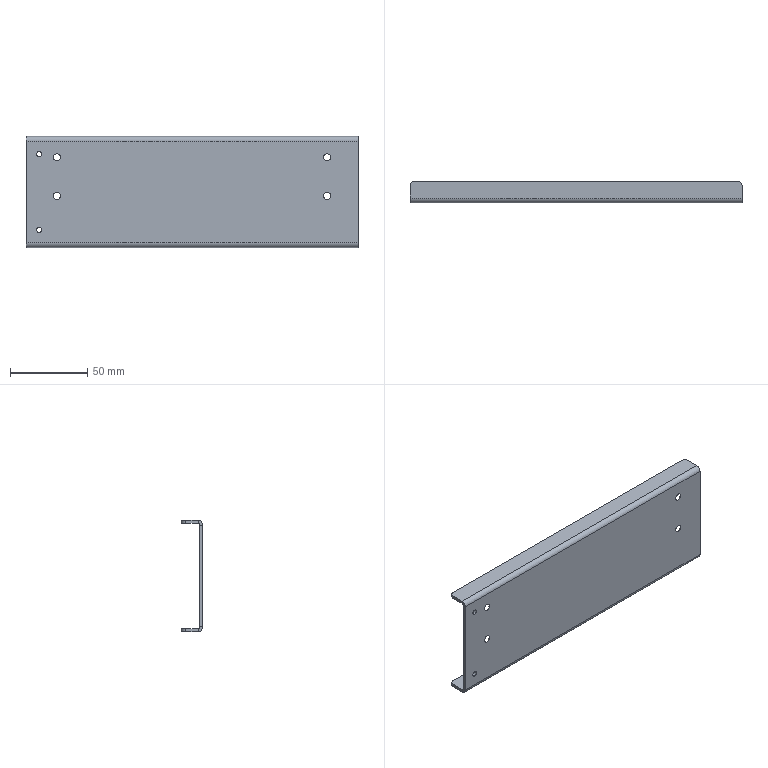Part | SolidWorks | features HoleWzd 2, Fillet 1, FlatPattern 1, SMBaseFlange 1, SheetMetal 1 | 1 solid | 38 faces | box 215 x 14 x 72 mm | volume 40210 mm3 | plane 18 | cylinder 12 | cone 8 | commonest cylinder face diameters 6 x6 3.3 x4 2 x2
STEP:
#1=CARTESIAN_POINT('',(8.5,-2.,-26.15));
#2=VERTEX_POINT('',#1);
#3=CARTESIAN_POINT('',(8.5,-2.,-22.85));
#4=VERTEX_POINT('',#3);
#5=CARTESIAN_POINT('',(8.5,-2.,-24.5));
#6=DIRECTION('',(0.,1.,0.));
#7=DIRECTION('',(0.,0.,1.));
#8=AXIS2_PLACEMENT_3D('',#5,#6,#7);
#9=CIRCLE('',#8,1.65);
#10=EDGE_CURVE('',#2,#4,#9,.T.);
#11=ORIENTED_EDGE('',*,*,#10,.F.);
#12=CARTESIAN_POINT('',(8.5,0.,-26.15));
#13=VERTEX_POINT('',#12);
#14=CARTESIAN_POINT('',(8.5,0.,-26.15));
#15=DIRECTION('',(0.,1.,0.));
#16=VECTOR('',#15,1000.);
#17=LINE('',#14,#16);
#18=EDGE_CURVE('',#2,#13,#17,.T.);
#19=ORIENTED_EDGE('',*,*,#18,.T.);
#20=CARTESIAN_POINT('',(8.5,0.,-22.85));
#21=VERTEX_POINT('',#20);
#22=CARTESIAN_POINT('',(8.5,0.,-24.5));
#23=DIRECTION('',(0.,1.,0.));
#24=DIRECTION('',(0.,0.,1.));
#25=AXIS2_PLACEMENT_3D('',#22,#23,#24);
#26=CIRCLE('',#25,1.65);
#27=EDGE_CURVE('',#13,#21,#26,.T.);
#28=ORIENTED_EDGE('',*,*,#27,.T.);
#29=CARTESIAN_POINT('',(8.5,0.,-22.85));
#30=DIRECTION('',(0.,1.,0.));
#31=VECTOR('',#30,1000.);
#32=LINE('',#29,#31);
#33=EDGE_CURVE('',#4,#21,#32,.T.);
#34=ORIENTED_EDGE('',*,*,#33,.F.);
#35=EDGE_LOOP('',(#11,#19,#28,#34));
#36=FACE_OUTER_BOUND('',#35,.T.);
#37=CARTESIAN_POINT('',(8.5,0.,-24.5));
#38=DIRECTION('',(0.,1.,0.));
#39=DIRECTION('',(0.,0.,1.));
#40=AXIS2_PLACEMENT_3D('',#37,#38,#39);
#41=CYLINDRICAL_SURFACE('',#40,1.65);
#42=ADVANCED_FACE('',(#36),#41,.F.);
#43=CARTESIAN_POINT('',(8.5,-2.,22.85));
#44=VERTEX_POINT('',#43);
#45=CARTESIAN_POINT('',(8.5,-2.,26.15));
#46=VERTEX_POINT('',#45);
#47=CARTESIAN_POINT('',(8.5,-2.,24.5));
#48=DIRECTION('',(0.,1.,0.));
#49=DIRECTION('',(0.,0.,1.));
#50=AXIS2_PLACEMENT_3D('',#47,#48,#49);
#51=CIRCLE('',#50,1.65);
#52=EDGE_CURVE('',#44,#46,#51,.T.);
#53=ORIENTED_EDGE('',*,*,#52,.F.);
#54=CARTESIAN_POINT('',(8.5,0.,22.85));
#55=VERTEX_POINT('',#54);
#56=CARTESIAN_POINT('',(8.5,0.,22.85));
#57=DIRECTION('',(0.,1.,0.));
#58=VECTOR('',#57,1000.);
#59=LINE('',#56,#58);
#60=EDGE_CURVE('',#44,#55,#59,.T.);
#61=ORIENTED_EDGE('',*,*,#60,.T.);
#62=CARTESIAN_POINT('',(8.5,0.,26.15));
#63=VERTEX_POINT('',#62);
#64=CARTESIAN_POINT('',(8.5,0.,24.5));
#65=DIRECTION('',(0.,1.,0.));
#66=DIRECTION('',(0.,0.,1.));
#67=AXIS2_PLACEMENT_3D('',#64,#65,#66);
#68=CIRCLE('',#67,1.65);
#69=EDGE_CURVE('',#55,#63,#68,.T.);
#70=ORIENTED_EDGE('',*,*,#69,.T.);
#71=CARTESIAN_POINT('',(8.5,0.,26.15));
#72=DIRECTION('',(0.,1.,0.));
#73=VECTOR('',#72,1000.);
#74=LINE('',#71,#73);
#75=EDGE_CURVE('',#46,#63,#74,.T.);
#76=ORIENTED_EDGE('',*,*,#75,.F.);
#77=EDGE_LOOP('',(#53,#61,#70,#76));
#78=FACE_OUTER_BOUND('',#77,.T.);
#79=CARTESIAN_POINT('',(8.5,0.,24.5));
#80=DIRECTION('',(0.,1.,0.));
#81=DIRECTION('',(0.,0.,1.));
#82=AXIS2_PLACEMENT_3D('',#79,#80,#81);
#83=CYLINDRICAL_SURFACE('',#82,1.65);
#84=ADVANCED_FACE('',(#78),#83,.F.);
#85=CARTESIAN_POINT('',(20.,-2.,-4.8));
#86=VERTEX_POINT('',#85);
#87=CARTESIAN_POINT('',(20.,-2.,-0.2));
#88=VERTEX_POINT('',#87);
#89=CARTESIAN_POINT('',(20.,-2.,-2.5));
#90=DIRECTION('',(0.,1.,0.));
#91=DIRECTION('',(0.,0.,1.));
#92=AXIS2_PLACEMENT_3D('',#89,#90,#91);
#93=CIRCLE('',#92,2.3);
#94=EDGE_CURVE('',#86,#88,#93,.T.);
#95=ORIENTED_EDGE('',*,*,#94,.F.);
#96=CARTESIAN_POINT('',(20.,0.,-6.8));
#97=VERTEX_POINT('',#96);
#98=CARTESIAN_POINT('',(20.,0.,-6.8));
#99=DIRECTION('',(0.,0.7071,-0.7071));
#100=VECTOR('',#99,1000.);
#101=LINE('',#98,#100);
#102=EDGE_CURVE('',#86,#97,#101,.T.);
#103=ORIENTED_EDGE('',*,*,#102,.T.);
#104=CARTESIAN_POINT('',(20.,0.,1.8));
#105=VERTEX_POINT('',#104);
#106=CARTESIAN_POINT('',(20.,0.,-2.5));
#107=DIRECTION('',(0.,1.,0.));
#108=DIRECTION('',(0.,0.,1.));
#109=AXIS2_PLACEMENT_3D('',#106,#107,#108);
#110=CIRCLE('',#109,4.3);
#111=EDGE_CURVE('',#97,#105,#110,.T.);
#112=ORIENTED_EDGE('',*,*,#111,.T.);
#113=CARTESIAN_POINT('',(20.,0.,1.8));
#114=DIRECTION('',(0.,0.7071,0.7071));
#115=VECTOR('',#114,1000.);
#116=LINE('',#113,#115);
#117=EDGE_CURVE('',#88,#105,#116,.T.);
#118=ORIENTED_EDGE('',*,*,#117,.F.);
#119=EDGE_LOOP('',(#95,#103,#112,#118));
#120=FACE_OUTER_BOUND('',#119,.T.);
#121=CARTESIAN_POINT('',(20.,0.,-2.5));
#122=DIRECTION('',(0.,1.,0.));
#123=DIRECTION('',(0.,0.,1.));
#124=AXIS2_PLACEMENT_3D('',#121,#122,#123);
#125=CONICAL_SURFACE('',#124,4.3,0.7854);
#126=ADVANCED_FACE('',(#120),#125,.F.);
#127=CARTESIAN_POINT('',(20.,-2.,20.2));
#128=VERTEX_POINT('',#127);
#129=CARTESIAN_POINT('',(20.,-2.,24.8));
#130=VERTEX_POINT('',#129);
#131=CARTESIAN_POINT('',(20.,-2.,22.5));
#132=DIRECTION('',(0.,1.,0.));
#133=DIRECTION('',(0.,0.,1.));
#134=AXIS2_PLACEMENT_3D('',#131,#132,#133);
#135=CIRCLE('',#134,2.3);
#136=EDGE_CURVE('',#128,#130,#135,.T.);
#137=ORIENTED_EDGE('',*,*,#136,.F.);
#138=CARTESIAN_POINT('',(20.,0.,18.2));
#139=VERTEX_POINT('',#138);
#140=CARTESIAN_POINT('',(20.,0.,18.2));
#141=DIRECTION('',(0.,0.7071,-0.7071));
#142=VECTOR('',#141,1000.);
#143=LINE('',#140,#142);
#144=EDGE_CURVE('',#128,#139,#143,.T.);
#145=ORIENTED_EDGE('',*,*,#144,.T.);
#146=CARTESIAN_POINT('',(20.,0.,26.8));
#147=VERTEX_POINT('',#146);
#148=CARTESIAN_POINT('',(20.,0.,22.5));
#149=DIRECTION('',(0.,1.,0.));
#150=DIRECTION('',(0.,0.,1.));
#151=AXIS2_PLACEMENT_3D('',#148,#149,#150);
#152=CIRCLE('',#151,4.3);
#153=EDGE_CURVE('',#139,#147,#152,.T.);
#154=ORIENTED_EDGE('',*,*,#153,.T.);
#155=CARTESIAN_POINT('',(20.,0.,26.8));
#156=DIRECTION('',(0.,0.7071,0.7071));
#157=VECTOR('',#156,1000.);
#158=LINE('',#155,#157);
#159=EDGE_CURVE('',#130,#147,#158,.T.);
#160=ORIENTED_EDGE('',*,*,#159,.F.);
#161=EDGE_LOOP('',(#137,#145,#154,#160));
#162=FACE_OUTER_BOUND('',#161,.T.);
#163=CARTESIAN_POINT('',(20.,0.,22.5));
#164=DIRECTION('',(0.,1.,0.));
#165=DIRECTION('',(0.,0.,1.));
#166=AXIS2_PLACEMENT_3D('',#163,#164,#165);
#167=CONICAL_SURFACE('',#166,4.3,0.7854);
#168=ADVANCED_FACE('',(#162),#167,.F.);
#169=CARTESIAN_POINT('',(195.,-2.,20.2));
#170=VERTEX_POINT('',#169);
#171=CARTESIAN_POINT('',(195.,-2.,24.8));
#172=VERTEX_POINT('',#171);
#173=CARTESIAN_POINT('',(195.,-2.,22.5));
#174=DIRECTION('',(0.,1.,0.));
#175=DIRECTION('',(0.,0.,1.));
#176=AXIS2_PLACEMENT_3D('',#173,#174,#175);
#177=CIRCLE('',#176,2.3);
#178=EDGE_CURVE('',#170,#172,#177,.T.);
#179=ORIENTED_EDGE('',*,*,#178,.F.);
#180=CARTESIAN_POINT('',(195.,0.,18.2));
#181=VERTEX_POINT('',#180);
#182=CARTESIAN_POINT('',(195.,0.,18.2));
#183=DIRECTION('',(0.,0.7071,-0.7071));
#184=VECTOR('',#183,1000.);
#185=LINE('',#182,#184);
#186=EDGE_CURVE('',#170,#181,#185,.T.);
#187=ORIENTED_EDGE('',*,*,#186,.T.);
#188=CARTESIAN_POINT('',(195.,0.,26.8));
#189=VERTEX_POINT('',#188);
#190=CARTESIAN_POINT('',(195.,0.,22.5));
#191=DIRECTION('',(0.,1.,0.));
#192=DIRECTION('',(0.,0.,1.));
#193=AXIS2_PLACEMENT_3D('',#190,#191,#192);
#194=CIRCLE('',#193,4.3);
#195=EDGE_CURVE('',#181,#189,#194,.T.);
#196=ORIENTED_EDGE('',*,*,#195,.T.);
#197=CARTESIAN_POINT('',(195.,0.,26.8));
#198=DIRECTION('',(0.,0.7071,0.7071));
#199=VECTOR('',#198,1000.);
#200=LINE('',#197,#199);
#201=EDGE_CURVE('',#172,#189,#200,.T.);
#202=ORIENTED_EDGE('',*,*,#201,.F.);
#203=EDGE_LOOP('',(#179,#187,#196,#202));
#204=FACE_OUTER_BOUND('',#203,.T.);
#205=CARTESIAN_POINT('',(195.,0.,22.5));
#206=DIRECTION('',(0.,1.,0.));
#207=DIRECTION('',(0.,0.,1.));
#208=AXIS2_PLACEMENT_3D('',#205,#206,#207);
#209=CONICAL_SURFACE('',#208,4.3,0.7854);
#210=ADVANCED_FACE('',(#204),#209,.F.);
#211=CARTESIAN_POINT('',(195.,-2.,-4.8));
#212=VERTEX_POINT('',#211);
#213=CARTESIAN_POINT('',(195.,-2.,-0.2));
#214=VERTEX_POINT('',#213);
#215=CARTESIAN_POINT('',(195.,-2.,-2.5));
#216=DIRECTION('',(0.,1.,0.));
#217=DIRECTION('',(0.,0.,1.));
#218=AXIS2_PLACEMENT_3D('',#215,#216,#217);
#219=CIRCLE('',#218,2.3);
#220=EDGE_CURVE('',#212,#214,#219,.T.);
#221=ORIENTED_EDGE('',*,*,#220,.F.);
#222=CARTESIAN_POINT('',(195.,0.,-6.8));
#223=VERTEX_POINT('',#222);
#224=CARTESIAN_POINT('',(195.,0.,-6.8));
#225=DIRECTION('',(0.,0.7071,-0.7071));
#226=VECTOR('',#225,1000.);
#227=LINE('',#224,#226);
#228=EDGE_CURVE('',#212,#223,#227,.T.);
#229=ORIENTED_EDGE('',*,*,#228,.T.);
#230=CARTESIAN_POINT('',(195.,0.,1.8));
#231=VERTEX_POINT('',#230);
#232=CARTESIAN_POINT('',(195.,0.,-2.5));
#233=DIRECTION('',(0.,1.,0.));
#234=DIRECTION('',(0.,0.,1.));
#235=AXIS2_PLACEMENT_3D('',#232,#233,#234);
#236=CIRCLE('',#235,4.3);
#237=EDGE_CURVE('',#223,#231,#236,.T.);
#238=ORIENTED_EDGE('',*,*,#237,.T.);
#239=CARTESIAN_POINT('',(195.,0.,1.8));
#240=DIRECTION('',(0.,0.7071,0.7071));
#241=VECTOR('',#240,1000.);
#242=LINE('',#239,#241);
#243=EDGE_CURVE('',#214,#231,#242,.T.);
#244=ORIENTED_EDGE('',*,*,#243,.F.);
#245=EDGE_LOOP('',(#221,#229,#238,#244));
#246=FACE_OUTER_BOUND('',#245,.T.);
#247=CARTESIAN_POINT('',(195.,0.,-2.5));
#248=DIRECTION('',(0.,1.,0.));
#249=DIRECTION('',(0.,0.,1.));
#250=AXIS2_PLACEMENT_3D('',#247,#248,#249);
#251=CONICAL_SURFACE('',#250,4.3,0.7854);
#252=ADVANCED_FACE('',(#246),#251,.F.);
#253=CARTESIAN_POINT('',(215.,0.,33.));
#254=VERTEX_POINT('',#253);
#255=CARTESIAN_POINT('',(215.,-2.,33.));
#256=VERTEX_POINT('',#255);
#257=CARTESIAN_POINT('',(215.,0.,33.));
#258=DIRECTION('',(0.,-1.,0.));
#259=VECTOR('',#258,1000.);
#260=LINE('',#257,#259);
#261=EDGE_CURVE('',#254,#256,#260,.T.);
#262=ORIENTED_EDGE('',*,*,#261,.F.);
#263=CARTESIAN_POINT('',(215.,1.,34.));
#264=VERTEX_POINT('',#263);
#265=CARTESIAN_POINT('',(215.,1.,33.));
#266=DIRECTION('',(1.,0.,0.));
#267=DIRECTION('',(0.,0.,1.));
#268=AXIS2_PLACEMENT_3D('',#265,#266,#267);
#269=CIRCLE('',#268,1.);
#270=EDGE_CURVE('',#264,#254,#269,.T.);
#271=ORIENTED_EDGE('',*,*,#270,.F.);
#272=CARTESIAN_POINT('',(215.,1.,36.));
#273=VERTEX_POINT('',#272);
#274=CARTESIAN_POINT('',(215.,1.,36.));
#275=DIRECTION('',(0.,0.,-1.));
#276=VECTOR('',#275,1000.);
#277=LINE('',#274,#276);
#278=EDGE_CURVE('',#273,#264,#277,.T.);
#279=ORIENTED_EDGE('',*,*,#278,.F.);
#280=CARTESIAN_POINT('',(215.,1.,33.));
#281=DIRECTION('',(1.,0.,0.));
#282=DIRECTION('',(0.,0.,-1.));
#283=AXIS2_PLACEMENT_3D('',#280,#281,#282);
#284=CIRCLE('',#283,3.);
#285=EDGE_CURVE('',#273,#256,#284,.T.);
#286=ORIENTED_EDGE('',*,*,#285,.T.);
#287=EDGE_LOOP('',(#262,#271,#279,#286));
#288=FACE_OUTER_BOUND('',#287,.T.);
#289=CARTESIAN_POINT('',(215.,0.,33.));
#290=DIRECTION('',(1.,0.,0.));
#291=DIRECTION('',(0.,0.,-1.));
#292=AXIS2_PLACEMENT_3D('',#289,#290,#291);
#293=PLANE('',#292);
#294=ADVANCED_FACE('',(#288),#293,.T.);
#295=CARTESIAN_POINT('',(215.,0.,-33.));
#296=VERTEX_POINT('',#295);
#297=CARTESIAN_POINT('',(215.,0.,34.));
#298=DIRECTION('',(0.,0.,-1.));
#299=VECTOR('',#298,1000.);
#300=LINE('',#297,#299);
#301=EDGE_CURVE('',#254,#296,#300,.T.);
#302=ORIENTED_EDGE('',*,*,#301,.F.);
#303=ORIENTED_EDGE('',*,*,#261,.T.);
#304=CARTESIAN_POINT('',(215.,-2.,-33.));
#305=VERTEX_POINT('',#304);
#306=CARTESIAN_POINT('',(215.,-2.,34.));
#307=DIRECTION('',(0.,0.,-1.));
#308=VECTOR('',#307,1000.);
#309=LINE('',#306,#308);
#310=EDGE_CURVE('',#256,#305,#309,.T.);
#311=ORIENTED_EDGE('',*,*,#310,.T.);
#312=CARTESIAN_POINT('',(215.,-2.,-33.));
#313=DIRECTION('',(0.,1.,0.));
#314=VECTOR('',#313,1000.);
#315=LINE('',#312,#314);
#316=EDGE_CURVE('',#305,#296,#315,.T.);
#317=ORIENTED_EDGE('',*,*,#316,.T.);
#318=EDGE_LOOP('',(#302,#303,#311,#317));
#319=FACE_OUTER_BOUND('',#318,.T.);
#320=CARTESIAN_POINT('',(215.,1.,36.));
#321=DIRECTION('',(1.,0.,0.));
#322=DIRECTION('',(0.,0.,-1.));
#323=AXIS2_PLACEMENT_3D('',#320,#321,#322);
#324=PLANE('',#323);
#325=ADVANCED_FACE('',(#319),#324,.T.);
#326=CARTESIAN_POINT('',(0.,1.,34.));
#327=VERTEX_POINT('',#326);
#328=CARTESIAN_POINT('',(0.,1.,36.));
#329=VERTEX_POINT('',#328);
#330=CARTESIAN_POINT('',(0.,1.,34.));
#331=DIRECTION('',(0.,0.,1.));
#332=VECTOR('',#331,1000.);
#333=LINE('',#330,#332);
#334=EDGE_CURVE('',#327,#329,#333,.T.);
#335=ORIENTED_EDGE('',*,*,#334,.F.);
#336=CARTESIAN_POINT('',(0.,0.,33.));
#337=VERTEX_POINT('',#336);
#338=CARTESIAN_POINT('',(0.,1.,33.));
#339=DIRECTION('',(1.,0.,0.));
#340=DIRECTION('',(0.,0.,1.));
#341=AXIS2_PLACEMENT_3D('',#338,#339,#340);
#342=CIRCLE('',#341,1.);
#343=EDGE_CURVE('',#327,#337,#342,.T.);
#344=ORIENTED_EDGE('',*,*,#343,.T.);
#345=CARTESIAN_POINT('',(0.,-2.,33.));
#346=VERTEX_POINT('',#345);
#347=CARTESIAN_POINT('',(0.,-2.,33.));
#348=DIRECTION('',(0.,1.,0.));
#349=VECTOR('',#348,1000.);
#350=LINE('',#347,#349);
#351=EDGE_CURVE('',#346,#337,#350,.T.);
#352=ORIENTED_EDGE('',*,*,#351,.F.);
#353=CARTESIAN_POINT('',(0.,1.,33.));
#354=DIRECTION('',(1.,0.,0.));
#355=DIRECTION('',(0.,0.,-1.));
#356=AXIS2_PLACEMENT_3D('',#353,#354,#355);
#357=CIRCLE('',#356,3.);
#358=EDGE_CURVE('',#329,#346,#357,.T.);
#359=ORIENTED_EDGE('',*,*,#358,.F.);
#360=EDGE_LOOP('',(#335,#344,#352,#359));
#361=FACE_OUTER_BOUND('',#360,.T.);
#362=CARTESIAN_POINT('',(0.,1.,34.));
#363=DIRECTION('',(-1.,0.,0.));
#364=DIRECTION('',(0.,0.,1.));
#365=AXIS2_PLACEMENT_3D('',#362,#363,#364);
#366=PLANE('',#365);
#367=ADVANCED_FACE('',(#361),#366,.T.);
#368=CARTESIAN_POINT('',(0.,9.,36.));
#369=VERTEX_POINT('',#368);
#370=CARTESIAN_POINT('',(0.,0.,36.));
#371=DIRECTION('',(0.,-1.,0.));
#372=VECTOR('',#371,1000.);
#373=LINE('',#370,#372);
#374=EDGE_CURVE('',#369,#329,#373,.T.);
#375=ORIENTED_EDGE('',*,*,#374,.F.);
#376=CARTESIAN_POINT('',(0.,9.,34.));
#377=VERTEX_POINT('',#376);
#378=CARTESIAN_POINT('',(0.,9.,33.));
#379=DIRECTION('',(0.,0.,-1.));
#380=VECTOR('',#379,1000.);
#381=LINE('',#378,#380);
#382=EDGE_CURVE('',#369,#377,#381,.T.);
#383=ORIENTED_EDGE('',*,*,#382,.T.);
#384=CARTESIAN_POINT('',(0.,0.,34.));
#385=DIRECTION('',(0.,-1.,0.));
#386=VECTOR('',#385,1000.);
#387=LINE('',#384,#386);
#388=EDGE_CURVE('',#377,#327,#387,.T.);
#389=ORIENTED_EDGE('',*,*,#388,.T.);
#390=ORIENTED_EDGE('',*,*,#334,.T.);
#391=EDGE_LOOP('',(#375,#383,#389,#390));
#392=FACE_OUTER_BOUND('',#391,.T.);
#393=CARTESIAN_POINT('',(0.,-2.,33.));
#394=DIRECTION('',(-1.,0.,0.));
#395=DIRECTION('',(0.,0.,1.));
#396=AXIS2_PLACEMENT_3D('',#393,#394,#395);
#397=PLANE('',#396);
#398=ADVANCED_FACE('',(#392),#397,.T.);
#399=CARTESIAN_POINT('',(215.,1.,-34.));
#400=VERTEX_POINT('',#399);
#401=CARTESIAN_POINT('',(215.,1.,-36.));
#402=VERTEX_POINT('',#401);
#403=CARTESIAN_POINT('',(215.,1.,-34.));
#404=DIRECTION('',(0.,0.,-1.));
#405=VECTOR('',#404,1000.);
#406=LINE('',#403,#405);
#407=EDGE_CURVE('',#400,#402,#406,.T.);
#408=ORIENTED_EDGE('',*,*,#407,.F.);
#409=CARTESIAN_POINT('',(215.,1.,-33.));
#410=DIRECTION('',(1.,0.,0.));
#411=DIRECTION('',(0.,0.,1.));
#412=AXIS2_PLACEMENT_3D('',#409,#410,#411);
#413=CIRCLE('',#412,1.);
#414=EDGE_CURVE('',#296,#400,#413,.T.);
#415=ORIENTED_EDGE('',*,*,#414,.F.);
#416=ORIENTED_EDGE('',*,*,#316,.F.);
#417=CARTESIAN_POINT('',(215.,1.,-33.));
#418=DIRECTION('',(1.,0.,0.));
#419=DIRECTION('',(0.,0.,-1.));
#420=AXIS2_PLACEMENT_3D('',#417,#418,#419);
#421=CIRCLE('',#420,3.);
#422=EDGE_CURVE('',#305,#402,#421,.T.);
#423=ORIENTED_EDGE('',*,*,#422,.T.);
#424=EDGE_LOOP('',(#408,#415,#416,#423));
#425=FACE_OUTER_BOUND('',#424,.T.);
#426=CARTESIAN_POINT('',(215.,1.,-34.));
#427=DIRECTION('',(1.,0.,0.));
#428=DIRECTION('',(0.,0.,-1.));
#429=AXIS2_PLACEMENT_3D('',#426,#427,#428);
#430=PLANE('',#429);
#431=ADVANCED_FACE('',(#425),#430,.T.);
#432=CARTESIAN_POINT('',(215.,9.,-36.));
#433=VERTEX_POINT('',#432);
#434=CARTESIAN_POINT('',(215.,0.,-36.));
#435=DIRECTION('',(0.,1.,0.));
#436=VECTOR('',#435,1000.);
#437=LINE('',#434,#436);
#438=EDGE_CURVE('',#402,#433,#437,.T.);
#439=ORIENTED_EDGE('',*,*,#438,.T.);
#440=CARTESIAN_POINT('',(215.,9.,-34.));
#441=VERTEX_POINT('',#440);
#442=CARTESIAN_POINT('',(215.,9.,-33.));
#443=DIRECTION('',(0.,0.,1.));
#444=VECTOR('',#443,1000.);
#445=LINE('',#442,#444);
#446=EDGE_CURVE('',#433,#441,#445,.T.);
#447=ORIENTED_EDGE('',*,*,#446,.T.);
#448=CARTESIAN_POINT('',(215.,0.,-34.));
#449=DIRECTION('',(0.,1.,0.));
#450=VECTOR('',#449,1000.);
#451=LINE('',#448,#450);
#452=EDGE_CURVE('',#400,#441,#451,.T.);
#453=ORIENTED_EDGE('',*,*,#452,.F.);
#454=ORIENTED_EDGE('',*,*,#407,.T.);
#455=EDGE_LOOP('',(#439,#447,#453,#454));
#456=FACE_OUTER_BOUND('',#455,.T.);
#457=CARTESIAN_POINT('',(215.,-2.,-33.));
#458=DIRECTION('',(1.,0.,0.));
#459=DIRECTION('',(0.,0.,-1.));
#460=AXIS2_PLACEMENT_3D('',#457,#458,#459);
#461=PLANE('',#460);
#462=ADVANCED_FACE('',(#456),#461,.T.);
#463=CARTESIAN_POINT('',(0.,0.,-33.));
#464=VERTEX_POINT('',#463);
#465=CARTESIAN_POINT('',(0.,-2.,-33.));
#466=VERTEX_POINT('',#465);
#467=CARTESIAN_POINT('',(0.,0.,-33.));
#468=DIRECTION('',(0.,-1.,0.));
#469=VECTOR('',#468,1000.);
#470=LINE('',#467,#469);
#471=EDGE_CURVE('',#464,#466,#470,.T.);
#472=ORIENTED_EDGE('',*,*,#471,.F.);
#473=CARTESIAN_POINT('',(0.,1.,-34.));
#474=VERTEX_POINT('',#473);
#475=CARTESIAN_POINT('',(0.,1.,-33.));
#476=DIRECTION('',(1.,0.,0.));
#477=DIRECTION('',(0.,0.,1.));
#478=AXIS2_PLACEMENT_3D('',#475,#476,#477);
#479=CIRCLE('',#478,1.);
#480=EDGE_CURVE('',#464,#474,#479,.T.);
#481=ORIENTED_EDGE('',*,*,#480,.T.);
#482=CARTESIAN_POINT('',(0.,1.,-36.));
#483=VERTEX_POINT('',#482);
#484=CARTESIAN_POINT('',(0.,1.,-36.));
#485=DIRECTION('',(0.,0.,1.));
#486=VECTOR('',#485,1000.);
#487=LINE('',#484,#486);
#488=EDGE_CURVE('',#483,#474,#487,.T.);
#489=ORIENTED_EDGE('',*,*,#488,.F.);
#490=CARTESIAN_POINT('',(0.,1.,-33.));
#491=DIRECTION('',(1.,0.,0.));
#492=DIRECTION('',(0.,0.,-1.));
#493=AXIS2_PLACEMENT_3D('',#490,#491,#492);
#494=CIRCLE('',#493,3.);
#495=EDGE_CURVE('',#466,#483,#494,.T.);
#496=ORIENTED_EDGE('',*,*,#495,.F.);
#497=EDGE_LOOP('',(#472,#481,#489,#496));
#498=FACE_OUTER_BOUND('',#497,.T.);
#499=CARTESIAN_POINT('',(0.,0.,-33.));
#500=DIRECTION('',(-1.,0.,0.));
#501=DIRECTION('',(0.,0.,1.));
#502=AXIS2_PLACEMENT_3D('',#499,#500,#501);
#503=PLANE('',#502);
#504=ADVANCED_FACE('',(#498),#503,.T.);
#505=CARTESIAN_POINT('',(0.,0.,34.));
#506=DIRECTION('',(0.,0.,-1.));
#507=VECTOR('',#506,1000.);
#508=LINE('',#505,#507);
#509=EDGE_CURVE('',#337,#464,#508,.T.);
#510=ORIENTED_EDGE('',*,*,#509,.T.);
#511=ORIENTED_EDGE('',*,*,#471,.T.);
#512=CARTESIAN_POINT('',(0.,-2.,34.));
#513=DIRECTION('',(0.,0.,-1.));
#514=VECTOR('',#513,1000.);
#515=LINE('',#512,#514);
#516=EDGE_CURVE('',#346,#466,#515,.T.);
#517=ORIENTED_EDGE('',*,*,#516,.F.);
#518=ORIENTED_EDGE('',*,*,#351,.T.);
#519=EDGE_LOOP('',(#510,#511,#517,#518));
#520=FACE_OUTER_BOUND('',#519,.T.);
#521=CARTESIAN_POINT('',(0.,1.,-36.));
#522=DIRECTION('',(-1.,0.,0.));
#523=DIRECTION('',(0.,0.,1.));
#524=AXIS2_PLACEMENT_3D('',#521,#522,#523);
#525=PLANE('',#524);
#526=ADVANCED_FACE('',(#520),#525,.T.);
#527=CARTESIAN_POINT('',(212.,12.,-36.));
#528=VERTEX_POINT('',#527);
#529=CARTESIAN_POINT('',(3.,12.,-36.));
#530=VERTEX_POINT('',#529);
#531=CARTESIAN_POINT('',(215.,12.,-36.));
#532=DIRECTION('',(-1.,0.,0.));
#533=VECTOR('',#532,1000.);
#534=LINE('',#531,#533);
#535=EDGE_CURVE('',#528,#530,#534,.T.);
#536=ORIENTED_EDGE('',*,*,#535,.F.);
#537=CARTESIAN_POINT('',(212.,9.,-36.));
#538=DIRECTION('',(0.,0.,-1.));
#539=DIRECTION('',(1.,0.,0.));
#540=AXIS2_PLACEMENT_3D('',#537,#538,#539);
#541=CIRCLE('',#540,3.);
#542=EDGE_CURVE('',#528,#433,#541,.T.);
#543=ORIENTED_EDGE('',*,*,#542,.T.);
#544=ORIENTED_EDGE('',*,*,#438,.F.);
#545=CARTESIAN_POINT('',(215.,1.,-36.));
#546=DIRECTION('',(-1.,0.,0.));
#547=VECTOR('',#546,1000.);
#548=LINE('',#545,#547);
#549=EDGE_CURVE('',#402,#483,#548,.T.);
#550=ORIENTED_EDGE('',*,*,#549,.T.);
#551=CARTESIAN_POINT('',(0.,9.,-36.));
#552=VERTEX_POINT('',#551);
#553=CARTESIAN_POINT('',(0.,0.,-36.));
#554=DIRECTION('',(0.,1.,0.));
#555=VECTOR('',#554,1000.);
#556=LINE('',#553,#555);
#557=EDGE_CURVE('',#483,#552,#556,.T.);
#558=ORIENTED_EDGE('',*,*,#557,.T.);
#559=CARTESIAN_POINT('',(3.,9.,-36.));
#560=DIRECTION('',(0.,0.,-1.));
#561=DIRECTION('',(1.,0.,0.));
#562=AXIS2_PLACEMENT_3D('',#559,#560,#561);
#563=CIRCLE('',#562,3.);
#564=EDGE_CURVE('',#552,#530,#563,.T.);
#565=ORIENTED_EDGE('',*,*,#564,.T.);
#566=EDGE_LOOP('',(#536,#543,#544,#550,#558,#565));
#567=FACE_OUTER_BOUND('',#566,.T.);
#568=CARTESIAN_POINT('',(215.,0.,-36.));
#569=DIRECTION('',(0.,0.,1.));
#570=DIRECTION('',(1.,0.,0.));
#571=AXIS2_PLACEMENT_3D('',#568,#569,#570);
#572=PLANE('',#571);
#573=ADVANCED_FACE('',(#567),#572,.F.);
#574=CARTESIAN_POINT('',(212.,12.,-34.));
#575=VERTEX_POINT('',#574);
#576=CARTESIAN_POINT('',(3.,12.,-34.));
#577=VERTEX_POINT('',#576);
#578=CARTESIAN_POINT('',(215.,12.,-34.));
#579=DIRECTION('',(-1.,0.,0.));
#580=VECTOR('',#579,1000.);
#581=LINE('',#578,#580);
#582=EDGE_CURVE('',#575,#577,#581,.T.);
#583=ORIENTED_EDGE('',*,*,#582,.F.);
#584=CARTESIAN_POINT('',(212.,12.,-34.));
#585=DIRECTION('',(0.,0.,-1.));
#586=VECTOR('',#585,1000.);
#587=LINE('',#584,#586);
#588=EDGE_CURVE('',#575,#528,#587,.T.);
#589=ORIENTED_EDGE('',*,*,#588,.T.);
#590=ORIENTED_EDGE('',*,*,#535,.T.);
#591=CARTESIAN_POINT('',(3.,12.,-34.));
#592=DIRECTION('',(0.,0.,1.));
#593=VECTOR('',#592,1000.);
#594=LINE('',#591,#593);
#595=EDGE_CURVE('',#530,#577,#594,.T.);
#596=ORIENTED_EDGE('',*,*,#595,.T.);
#597=EDGE_LOOP('',(#583,#589,#590,#596));
#598=FACE_OUTER_BOUND('',#597,.T.);
#599=CARTESIAN_POINT('',(215.,12.,-34.));
#600=DIRECTION('',(0.,1.,0.));
#601=DIRECTION('',(0.,0.,1.));
#602=AXIS2_PLACEMENT_3D('',#599,#600,#601);
#603=PLANE('',#602);
#604=ADVANCED_FACE('',(#598),#603,.T.);
#605=ORIENTED_EDGE('',*,*,#452,.T.);
#606=CARTESIAN_POINT('',(212.,9.,-34.));
#607=DIRECTION('',(0.,0.,1.));
#608=DIRECTION('',(1.,0.,0.));
#609=AXIS2_PLACEMENT_3D('',#606,#607,#608);
#610=CIRCLE('',#609,3.);
#611=EDGE_CURVE('',#441,#575,#610,.T.);
#612=ORIENTED_EDGE('',*,*,#611,.T.);
#613=ORIENTED_EDGE('',*,*,#582,.T.);
#614=CARTESIAN_POINT('',(0.,9.,-34.));
#615=VERTEX_POINT('',#614);
#616=CARTESIAN_POINT('',(3.,9.,-34.));
#617=DIRECTION('',(0.,0.,1.));
#618=DIRECTION('',(1.,0.,0.));
#619=AXIS2_PLACEMENT_3D('',#616,#617,#618);
#620=CIRCLE('',#619,3.);
#621=EDGE_CURVE('',#577,#615,#620,.T.);
#622=ORIENTED_EDGE('',*,*,#621,.T.);
#623=CARTESIAN_POINT('',(0.,0.,-34.));
#624=DIRECTION('',(0.,1.,0.));
#625=VECTOR('',#624,1000.);
#626=LINE('',#623,#625);
#627=EDGE_CURVE('',#474,#615,#626,.T.);
#628=ORIENTED_EDGE('',*,*,#627,.F.);
#629=CARTESIAN_POINT('',(215.,1.,-34.));
#630=DIRECTION('',(-1.,0.,0.));
#631=VECTOR('',#630,1000.);
#632=LINE('',#629,#631);
#633=EDGE_CURVE('',#400,#474,#632,.T.);
#634=ORIENTED_EDGE('',*,*,#633,.F.);
#635=EDGE_LOOP('',(#605,#612,#613,#622,#628,#634));
#636=FACE_OUTER_BOUND('',#635,.T.);
#637=CARTESIAN_POINT('',(215.,0.,-34.));
#638=DIRECTION('',(0.,0.,1.));
#639=DIRECTION('',(1.,0.,0.));
#640=AXIS2_PLACEMENT_3D('',#637,#638,#639);
#641=PLANE('',#640);
#642=ADVANCED_FACE('',(#636),#641,.T.);
#643=ORIENTED_EDGE('',*,*,#480,.F.);
#644=CARTESIAN_POINT('',(215.,0.,-33.));
#645=DIRECTION('',(-1.,0.,0.));
#646=VECTOR('',#645,1000.);
#647=LINE('',#644,#646);
#648=EDGE_CURVE('',#296,#464,#647,.T.);
#649=ORIENTED_EDGE('',*,*,#648,.F.);
#650=ORIENTED_EDGE('',*,*,#414,.T.);
#651=ORIENTED_EDGE('',*,*,#633,.T.);
#652=EDGE_LOOP('',(#643,#649,#650,#651));
#653=FACE_OUTER_BOUND('',#652,.T.);
#654=CARTESIAN_POINT('',(215.,1.,-33.));
#655=DIRECTION('',(-1.,0.,0.));
#656=DIRECTION('',(0.,0.,1.));
#657=AXIS2_PLACEMENT_3D('',#654,#655,#656);
#658=CYLINDRICAL_SURFACE('',#657,1.);
#659=ADVANCED_FACE('',(#653),#658,.F.);
#660=CARTESIAN_POINT('',(8.5,0.,-24.5));
#661=DIRECTION('',(0.,1.,0.));
#662=DIRECTION('',(0.,0.,1.));
#663=AXIS2_PLACEMENT_3D('',#660,#661,#662);
#664=CIRCLE('',#663,1.65);
#665=EDGE_CURVE('',#21,#13,#664,.T.);
#666=ORIENTED_EDGE('',*,*,#665,.F.);
#667=ORIENTED_EDGE('',*,*,#27,.F.);
#668=EDGE_LOOP('',(#666,#667));
#669=FACE_BOUND('',#668,.T.);
#670=CARTESIAN_POINT('',(8.5,0.,24.5));
#671=DIRECTION('',(0.,1.,0.));
#672=DIRECTION('',(0.,0.,1.));
#673=AXIS2_PLACEMENT_3D('',#670,#671,#672);
#674=CIRCLE('',#673,1.65);
#675=EDGE_CURVE('',#63,#55,#674,.T.);
#676=ORIENTED_EDGE('',*,*,#675,.F.);
#677=ORIENTED_EDGE('',*,*,#69,.F.);
#678=EDGE_LOOP('',(#676,#677));
#679=FACE_BOUND('',#678,.T.);
#680=CARTESIAN_POINT('',(20.,0.,-2.5));
#681=DIRECTION('',(0.,1.,0.));
#682=DIRECTION('',(0.,0.,1.));
#683=AXIS2_PLACEMENT_3D('',#680,#681,#682);
#684=CIRCLE('',#683,4.3);
#685=EDGE_CURVE('',#105,#97,#684,.T.);
#686=ORIENTED_EDGE('',*,*,#685,.F.);
#687=ORIENTED_EDGE('',*,*,#111,.F.);
#688=EDGE_LOOP('',(#686,#687));
#689=FACE_BOUND('',#688,.T.);
#690=CARTESIAN_POINT('',(20.,0.,22.5));
#691=DIRECTION('',(0.,1.,0.));
#692=DIRECTION('',(0.,0.,1.));
#693=AXIS2_PLACEMENT_3D('',#690,#691,#692);
#694=CIRCLE('',#693,4.3);
#695=EDGE_CURVE('',#147,#139,#694,.T.);
#696=ORIENTED_EDGE('',*,*,#695,.F.);
#697=ORIENTED_EDGE('',*,*,#153,.F.);
#698=EDGE_LOOP('',(#696,#697));
#699=FACE_BOUND('',#698,.T.);
#700=CARTESIAN_POINT('',(195.,0.,22.5));
#701=DIRECTION('',(0.,1.,0.));
#702=DIRECTION('',(0.,0.,1.));
#703=AXIS2_PLACEMENT_3D('',#700,#701,#702);
#704=CIRCLE('',#703,4.3);
#705=EDGE_CURVE('',#189,#181,#704,.T.);
#706=ORIENTED_EDGE('',*,*,#705,.F.);
#707=ORIENTED_EDGE('',*,*,#195,.F.);
#708=EDGE_LOOP('',(#706,#707));
#709=FACE_BOUND('',#708,.T.);
#710=CARTESIAN_POINT('',(195.,0.,-2.5));
#711=DIRECTION('',(0.,1.,0.));
#712=DIRECTION('',(0.,0.,1.));
#713=AXIS2_PLACEMENT_3D('',#710,#711,#712);
#714=CIRCLE('',#713,4.3);
#715=EDGE_CURVE('',#231,#223,#714,.T.);
#716=ORIENTED_EDGE('',*,*,#715,.F.);
#717=ORIENTED_EDGE('',*,*,#237,.F.);
#718=EDGE_LOOP('',(#716,#717));
#719=FACE_BOUND('',#718,.T.);
#720=ORIENTED_EDGE('',*,*,#509,.F.);
#721=CARTESIAN_POINT('',(215.,0.,33.));
#722=DIRECTION('',(-1.,0.,0.));
#723=VECTOR('',#722,1000.);
#724=LINE('',#721,#723);
#725=EDGE_CURVE('',#254,#337,#724,.T.);
#726=ORIENTED_EDGE('',*,*,#725,.F.);
#727=ORIENTED_EDGE('',*,*,#301,.T.);
#728=ORIENTED_EDGE('',*,*,#648,.T.);
#729=EDGE_LOOP('',(#720,#726,#727,#728));
#730=FACE_OUTER_BOUND('',#729,.T.);
#731=CARTESIAN_POINT('',(215.,0.,34.));
#732=DIRECTION('',(0.,1.,0.));
#733=DIRECTION('',(0.,0.,1.));
#734=AXIS2_PLACEMENT_3D('',#731,#732,#733);
#735=PLANE('',#734);
#736=ADVANCED_FACE('',(#669,#679,#689,#699,#709,#719,#730),#735,.T.);
#737=ORIENTED_EDGE('',*,*,#343,.F.);
#738=CARTESIAN_POINT('',(215.,1.,34.));
#739=DIRECTION('',(-1.,0.,0.));
#740=VECTOR('',#739,1000.);
#741=LINE('',#738,#740);
#742=EDGE_CURVE('',#264,#327,#741,.T.);
#743=ORIENTED_EDGE('',*,*,#742,.F.);
#744=ORIENTED_EDGE('',*,*,#270,.T.);
#745=ORIENTED_EDGE('',*,*,#725,.T.);
#746=EDGE_LOOP('',(#737,#743,#744,#745));
#747=FACE_OUTER_BOUND('',#746,.T.);
#748=CARTESIAN_POINT('',(215.,1.,33.));
#749=DIRECTION('',(-1.,0.,0.));
#750=DIRECTION('',(0.,0.,1.));
#751=AXIS2_PLACEMENT_3D('',#748,#749,#750);
#752=CYLINDRICAL_SURFACE('',#751,1.);
#753=ADVANCED_FACE('',(#747),#752,.F.);
#754=CARTESIAN_POINT('',(212.,12.,34.));
#755=VERTEX_POINT('',#754);
#756=CARTESIAN_POINT('',(3.,12.,34.));
#757=VERTEX_POINT('',#756);
#758=CARTESIAN_POINT('',(215.,12.,34.));
#759=DIRECTION('',(-1.,0.,0.));
#760=VECTOR('',#759,1000.);
#761=LINE('',#758,#760);
#762=EDGE_CURVE('',#755,#757,#761,.T.);
#763=ORIENTED_EDGE('',*,*,#762,.F.);
#764=CARTESIAN_POINT('',(215.,9.,34.));
#765=VERTEX_POINT('',#764);
#766=CARTESIAN_POINT('',(212.,9.,34.));
#767=DIRECTION('',(0.,0.,-1.));
#768=DIRECTION('',(-1.,0.,0.));
#769=AXIS2_PLACEMENT_3D('',#766,#767,#768);
#770=CIRCLE('',#769,3.);
#771=EDGE_CURVE('',#755,#765,#770,.T.);
#772=ORIENTED_EDGE('',*,*,#771,.T.);
#773=CARTESIAN_POINT('',(215.,0.,34.));
#774=DIRECTION('',(0.,-1.,0.));
#775=VECTOR('',#774,1000.);
#776=LINE('',#773,#775);
#777=EDGE_CURVE('',#765,#264,#776,.T.);
#778=ORIENTED_EDGE('',*,*,#777,.T.);
#779=ORIENTED_EDGE('',*,*,#742,.T.);
#780=ORIENTED_EDGE('',*,*,#388,.F.);
#781=CARTESIAN_POINT('',(3.,9.,34.));
#782=DIRECTION('',(0.,0.,-1.));
#783=DIRECTION('',(-1.,0.,0.));
#784=AXIS2_PLACEMENT_3D('',#781,#782,#783);
#785=CIRCLE('',#784,3.);
#786=EDGE_CURVE('',#377,#757,#785,.T.);
#787=ORIENTED_EDGE('',*,*,#786,.T.);
#788=EDGE_LOOP('',(#763,#772,#778,#779,#780,#787));
#789=FACE_OUTER_BOUND('',#788,.T.);
#790=CARTESIAN_POINT('',(215.,0.,34.));
#791=DIRECTION('',(0.,0.,-1.));
#792=DIRECTION('',(-1.,0.,0.));
#793=AXIS2_PLACEMENT_3D('',#790,#791,#792);
#794=PLANE('',#793);
#795=ADVANCED_FACE('',(#789),#794,.T.);
#796=CARTESIAN_POINT('',(212.,12.,36.));
#797=VERTEX_POINT('',#796);
#798=CARTESIAN_POINT('',(3.,12.,36.));
#799=VERTEX_POINT('',#798);
#800=CARTESIAN_POINT('',(215.,12.,36.));
#801=DIRECTION('',(-1.,0.,0.));
#802=VECTOR('',#801,1000.);
#803=LINE('',#800,#802);
#804=EDGE_CURVE('',#797,#799,#803,.T.);
#805=ORIENTED_EDGE('',*,*,#804,.F.);
#806=CARTESIAN_POINT('',(212.,12.,34.));
#807=DIRECTION('',(0.,0.,-1.));
#808=VECTOR('',#807,1000.);
#809=LINE('',#806,#808);
#810=EDGE_CURVE('',#797,#755,#809,.T.);
#811=ORIENTED_EDGE('',*,*,#810,.T.);
#812=ORIENTED_EDGE('',*,*,#762,.T.);
#813=CARTESIAN_POINT('',(3.,12.,36.));
#814=DIRECTION('',(0.,0.,1.));
#815=VECTOR('',#814,1000.);
#816=LINE('',#813,#815);
#817=EDGE_CURVE('',#757,#799,#816,.T.);
#818=ORIENTED_EDGE('',*,*,#817,.T.);
#819=EDGE_LOOP('',(#805,#811,#812,#818));
#820=FACE_OUTER_BOUND('',#819,.T.);
#821=CARTESIAN_POINT('',(215.,12.,36.));
#822=DIRECTION('',(0.,1.,0.));
#823=DIRECTION('',(0.,0.,1.));
#824=AXIS2_PLACEMENT_3D('',#821,#822,#823);
#825=PLANE('',#824);
#826=ADVANCED_FACE('',(#820),#825,.T.);
#827=CARTESIAN_POINT('',(215.,9.,36.));
#828=VERTEX_POINT('',#827);
#829=CARTESIAN_POINT('',(215.,0.,36.));
#830=DIRECTION('',(0.,-1.,0.));
#831=VECTOR('',#830,1000.);
#832=LINE('',#829,#831);
#833=EDGE_CURVE('',#828,#273,#832,.T.);
#834=ORIENTED_EDGE('',*,*,#833,.F.);
#835=CARTESIAN_POINT('',(212.,9.,36.));
#836=DIRECTION('',(0.,0.,1.));
#837=DIRECTION('',(-1.,0.,0.));
#838=AXIS2_PLACEMENT_3D('',#835,#836,#837);
#839=CIRCLE('',#838,3.);
#840=EDGE_CURVE('',#828,#797,#839,.T.);
#841=ORIENTED_EDGE('',*,*,#840,.T.);
#842=ORIENTED_EDGE('',*,*,#804,.T.);
#843=CARTESIAN_POINT('',(3.,9.,36.));
#844=DIRECTION('',(0.,0.,1.));
#845=DIRECTION('',(-1.,0.,0.));
#846=AXIS2_PLACEMENT_3D('',#843,#844,#845);
#847=CIRCLE('',#846,3.);
#848=EDGE_CURVE('',#799,#369,#847,.T.);
#849=ORIENTED_EDGE('',*,*,#848,.T.);
#850=ORIENTED_EDGE('',*,*,#374,.T.);
#851=CARTESIAN_POINT('',(215.,1.,36.));
#852=DIRECTION('',(-1.,0.,0.));
#853=VECTOR('',#852,1000.);
#854=LINE('',#851,#853);
#855=EDGE_CURVE('',#273,#329,#854,.T.);
#856=ORIENTED_EDGE('',*,*,#855,.F.);
#857=EDGE_LOOP('',(#834,#841,#842,#849,#850,#856));
#858=FACE_OUTER_BOUND('',#857,.T.);
#859=CARTESIAN_POINT('',(215.,0.,36.));
#860=DIRECTION('',(0.,0.,-1.));
#861=DIRECTION('',(-1.,0.,0.));
#862=AXIS2_PLACEMENT_3D('',#859,#860,#861);
#863=PLANE('',#862);
#864=ADVANCED_FACE('',(#858),#863,.F.);
#865=ORIENTED_EDGE('',*,*,#358,.T.);
#866=CARTESIAN_POINT('',(215.,-2.,33.));
#867=DIRECTION('',(-1.,0.,0.));
#868=VECTOR('',#867,1000.);
#869=LINE('',#866,#868);
#870=EDGE_CURVE('',#256,#346,#869,.T.);
#871=ORIENTED_EDGE('',*,*,#870,.F.);
#872=ORIENTED_EDGE('',*,*,#285,.F.);
#873=ORIENTED_EDGE('',*,*,#855,.T.);
#874=EDGE_LOOP('',(#865,#871,#872,#873));
#875=FACE_OUTER_BOUND('',#874,.T.);
#876=CARTESIAN_POINT('',(215.,1.,33.));
#877=DIRECTION('',(-1.,0.,0.));
#878=DIRECTION('',(0.,0.,1.));
#879=AXIS2_PLACEMENT_3D('',#876,#877,#878);
#880=CYLINDRICAL_SURFACE('',#879,3.);
#881=ADVANCED_FACE('',(#875),#880,.T.);
#882=CARTESIAN_POINT('',(8.5,-2.,-24.5));
#883=DIRECTION('',(0.,1.,0.));
#884=DIRECTION('',(0.,0.,1.));
#885=AXIS2_PLACEMENT_3D('',#882,#883,#884);
#886=CIRCLE('',#885,1.65);
#887=EDGE_CURVE('',#4,#2,#886,.T.);
#888=ORIENTED_EDGE('',*,*,#887,.T.);
#889=ORIENTED_EDGE('',*,*,#10,.T.);
#890=EDGE_LOOP('',(#888,#889));
#891=FACE_BOUND('',#890,.T.);
#892=CARTESIAN_POINT('',(8.5,-2.,24.5));
#893=DIRECTION('',(0.,1.,0.));
#894=DIRECTION('',(0.,0.,1.));
#895=AXIS2_PLACEMENT_3D('',#892,#893,#894);
#896=CIRCLE('',#895,1.65);
#897=EDGE_CURVE('',#46,#44,#896,.T.);
#898=ORIENTED_EDGE('',*,*,#897,.T.);
#899=ORIENTED_EDGE('',*,*,#52,.T.);
#900=EDGE_LOOP('',(#898,#899));
#901=FACE_BOUND('',#900,.T.);
#902=CARTESIAN_POINT('',(20.,-2.,-2.5));
#903=DIRECTION('',(0.,1.,0.));
#904=DIRECTION('',(0.,0.,1.));
#905=AXIS2_PLACEMENT_3D('',#902,#903,#904);
#906=CIRCLE('',#905,2.3);
#907=EDGE_CURVE('',#88,#86,#906,.T.);
#908=ORIENTED_EDGE('',*,*,#907,.T.);
#909=ORIENTED_EDGE('',*,*,#94,.T.);
#910=EDGE_LOOP('',(#908,#909));
#911=FACE_BOUND('',#910,.T.);
#912=CARTESIAN_POINT('',(20.,-2.,22.5));
#913=DIRECTION('',(0.,1.,0.));
#914=DIRECTION('',(0.,0.,1.));
#915=AXIS2_PLACEMENT_3D('',#912,#913,#914);
#916=CIRCLE('',#915,2.3);
#917=EDGE_CURVE('',#130,#128,#916,.T.);
#918=ORIENTED_EDGE('',*,*,#917,.T.);
#919=ORIENTED_EDGE('',*,*,#136,.T.);
#920=EDGE_LOOP('',(#918,#919));
#921=FACE_BOUND('',#920,.T.);
#922=CARTESIAN_POINT('',(195.,-2.,22.5));
#923=DIRECTION('',(0.,1.,0.));
#924=DIRECTION('',(0.,0.,1.));
#925=AXIS2_PLACEMENT_3D('',#922,#923,#924);
#926=CIRCLE('',#925,2.3);
#927=EDGE_CURVE('',#172,#170,#926,.T.);
#928=ORIENTED_EDGE('',*,*,#927,.T.);
#929=ORIENTED_EDGE('',*,*,#178,.T.);
#930=EDGE_LOOP('',(#928,#929));
#931=FACE_BOUND('',#930,.T.);
#932=CARTESIAN_POINT('',(195.,-2.,-2.5));
#933=DIRECTION('',(0.,1.,0.));
#934=DIRECTION('',(0.,0.,1.));
#935=AXIS2_PLACEMENT_3D('',#932,#933,#934);
#936=CIRCLE('',#935,2.3);
#937=EDGE_CURVE('',#214,#212,#936,.T.);
#938=ORIENTED_EDGE('',*,*,#937,.T.);
#939=ORIENTED_EDGE('',*,*,#220,.T.);
#940=EDGE_LOOP('',(#938,#939));
#941=FACE_BOUND('',#940,.T.);
#942=ORIENTED_EDGE('',*,*,#516,.T.);
#943=CARTESIAN_POINT('',(215.,-2.,-33.));
#944=DIRECTION('',(-1.,0.,0.));
#945=VECTOR('',#944,1000.);
#946=LINE('',#943,#945);
#947=EDGE_CURVE('',#305,#466,#946,.T.);
#948=ORIENTED_EDGE('',*,*,#947,.F.);
#949=ORIENTED_EDGE('',*,*,#310,.F.);
#950=ORIENTED_EDGE('',*,*,#870,.T.);
#951=EDGE_LOOP('',(#942,#948,#949,#950));
#952=FACE_OUTER_BOUND('',#951,.T.);
#953=CARTESIAN_POINT('',(215.,-2.,34.));
#954=DIRECTION('',(0.,1.,0.));
#955=DIRECTION('',(0.,0.,1.));
#956=AXIS2_PLACEMENT_3D('',#953,#954,#955);
#957=PLANE('',#956);
#958=ADVANCED_FACE('',(#891,#901,#911,#921,#931,#941,#952),#957,.F.);
#959=ORIENTED_EDGE('',*,*,#495,.T.);
#960=ORIENTED_EDGE('',*,*,#549,.F.);
#961=ORIENTED_EDGE('',*,*,#422,.F.);
#962=ORIENTED_EDGE('',*,*,#947,.T.);
#963=EDGE_LOOP('',(#959,#960,#961,#962));
#964=FACE_OUTER_BOUND('',#963,.T.);
#965=CARTESIAN_POINT('',(215.,1.,-33.));
#966=DIRECTION('',(-1.,0.,0.));
#967=DIRECTION('',(0.,0.,1.));
#968=AXIS2_PLACEMENT_3D('',#965,#966,#967);
#969=CYLINDRICAL_SURFACE('',#968,3.);
#970=ADVANCED_FACE('',(#964),#969,.T.);
#971=ORIENTED_EDGE('',*,*,#777,.F.);
#972=CARTESIAN_POINT('',(215.,9.,36.));
#973=DIRECTION('',(0.,0.,1.));
#974=VECTOR('',#973,1000.);
#975=LINE('',#972,#974);
#976=EDGE_CURVE('',#765,#828,#975,.T.);
#977=ORIENTED_EDGE('',*,*,#976,.T.);
#978=ORIENTED_EDGE('',*,*,#833,.T.);
#979=ORIENTED_EDGE('',*,*,#278,.T.);
#980=EDGE_LOOP('',(#971,#977,#978,#979));
#981=FACE_OUTER_BOUND('',#980,.T.);
#982=CARTESIAN_POINT('',(215.,1.,-33.));
#983=DIRECTION('',(-1.,0.,0.));
#984=DIRECTION('',(0.,0.,1.));
#985=AXIS2_PLACEMENT_3D('',#982,#983,#984);
#986=PLANE('',#985);
#987=ADVANCED_FACE('',(#981),#986,.F.);
#988=ORIENTED_EDGE('',*,*,#627,.T.);
#989=CARTESIAN_POINT('',(0.,9.,-33.));
#990=DIRECTION('',(0.,0.,-1.));
#991=VECTOR('',#990,1000.);
#992=LINE('',#989,#991);
#993=EDGE_CURVE('',#615,#552,#992,.T.);
#994=ORIENTED_EDGE('',*,*,#993,.T.);
#995=ORIENTED_EDGE('',*,*,#557,.F.);
#996=ORIENTED_EDGE('',*,*,#488,.T.);
#997=EDGE_LOOP('',(#988,#994,#995,#996));
#998=FACE_OUTER_BOUND('',#997,.T.);
#999=CARTESIAN_POINT('',(0.,1.,-33.));
#1000=DIRECTION('',(-1.,0.,0.));
#1001=DIRECTION('',(0.,0.,1.));
#1002=AXIS2_PLACEMENT_3D('',#999,#1000,#1001);
#1003=PLANE('',#1002);
#1004=ADVANCED_FACE('',(#998),#1003,.T.);
#1005=ORIENTED_EDGE('',*,*,#228,.F.);
#1006=ORIENTED_EDGE('',*,*,#937,.F.);
#1007=ORIENTED_EDGE('',*,*,#243,.T.);
#1008=ORIENTED_EDGE('',*,*,#715,.T.);
#1009=EDGE_LOOP('',(#1005,#1006,#1007,#1008));
#1010=FACE_OUTER_BOUND('',#1009,.T.);
#1011=CARTESIAN_POINT('',(195.,0.,-2.5));
#1012=DIRECTION('',(0.,1.,0.));
#1013=DIRECTION('',(0.,0.,1.));
#1014=AXIS2_PLACEMENT_3D('',#1011,#1012,#1013);
#1015=CONICAL_SURFACE('',#1014,4.3,0.7854);
#1016=ADVANCED_FACE('',(#1010),#1015,.F.);
#1017=ORIENTED_EDGE('',*,*,#186,.F.);
#1018=ORIENTED_EDGE('',*,*,#927,.F.);
#1019=ORIENTED_EDGE('',*,*,#201,.T.);
#1020=ORIENTED_EDGE('',*,*,#705,.T.);
#1021=EDGE_LOOP('',(#1017,#1018,#1019,#1020));
#1022=FACE_OUTER_BOUND('',#1021,.T.);
#1023=CARTESIAN_POINT('',(195.,0.,22.5));
#1024=DIRECTION('',(0.,1.,0.));
#1025=DIRECTION('',(0.,0.,1.));
#1026=AXIS2_PLACEMENT_3D('',#1023,#1024,#1025);
#1027=CONICAL_SURFACE('',#1026,4.3,0.7854);
#1028=ADVANCED_FACE('',(#1022),#1027,.F.);
#1029=ORIENTED_EDGE('',*,*,#144,.F.);
#1030=ORIENTED_EDGE('',*,*,#917,.F.);
#1031=ORIENTED_EDGE('',*,*,#159,.T.);
#1032=ORIENTED_EDGE('',*,*,#695,.T.);
#1033=EDGE_LOOP('',(#1029,#1030,#1031,#1032));
#1034=FACE_OUTER_BOUND('',#1033,.T.);
#1035=CARTESIAN_POINT('',(20.,0.,22.5));
#1036=DIRECTION('',(0.,1.,0.));
#1037=DIRECTION('',(0.,0.,1.));
#1038=AXIS2_PLACEMENT_3D('',#1035,#1036,#1037);
#1039=CONICAL_SURFACE('',#1038,4.3,0.7854);
#1040=ADVANCED_FACE('',(#1034),#1039,.F.);
#1041=ORIENTED_EDGE('',*,*,#102,.F.);
#1042=ORIENTED_EDGE('',*,*,#907,.F.);
#1043=ORIENTED_EDGE('',*,*,#117,.T.);
#1044=ORIENTED_EDGE('',*,*,#685,.T.);
#1045=EDGE_LOOP('',(#1041,#1042,#1043,#1044));
#1046=FACE_OUTER_BOUND('',#1045,.T.);
#1047=CARTESIAN_POINT('',(20.,0.,-2.5));
#1048=DIRECTION('',(0.,1.,0.));
#1049=DIRECTION('',(0.,0.,1.));
#1050=AXIS2_PLACEMENT_3D('',#1047,#1048,#1049);
#1051=CONICAL_SURFACE('',#1050,4.3,0.7854);
#1052=ADVANCED_FACE('',(#1046),#1051,.F.);
#1053=ORIENTED_EDGE('',*,*,#60,.F.);
#1054=ORIENTED_EDGE('',*,*,#897,.F.);
#1055=ORIENTED_EDGE('',*,*,#75,.T.);
#1056=ORIENTED_EDGE('',*,*,#675,.T.);
#1057=EDGE_LOOP('',(#1053,#1054,#1055,#1056));
#1058=FACE_OUTER_BOUND('',#1057,.T.);
#1059=CARTESIAN_POINT('',(8.5,0.,24.5));
#1060=DIRECTION('',(0.,1.,0.));
#1061=DIRECTION('',(0.,0.,1.));
#1062=AXIS2_PLACEMENT_3D('',#1059,#1060,#1061);
#1063=CYLINDRICAL_SURFACE('',#1062,1.65);
#1064=ADVANCED_FACE('',(#1058),#1063,.F.);
#1065=ORIENTED_EDGE('',*,*,#18,.F.);
#1066=ORIENTED_EDGE('',*,*,#887,.F.);
#1067=ORIENTED_EDGE('',*,*,#33,.T.);
#1068=ORIENTED_EDGE('',*,*,#665,.T.);
#1069=EDGE_LOOP('',(#1065,#1066,#1067,#1068));
#1070=FACE_OUTER_BOUND('',#1069,.T.);
#1071=CARTESIAN_POINT('',(8.5,0.,-24.5));
#1072=DIRECTION('',(0.,1.,0.));
#1073=DIRECTION('',(0.,0.,1.));
#1074=AXIS2_PLACEMENT_3D('',#1071,#1072,#1073);
#1075=CYLINDRICAL_SURFACE('',#1074,1.65);
#1076=ADVANCED_FACE('',(#1070),#1075,.F.);
#1077=ORIENTED_EDGE('',*,*,#840,.F.);
#1078=ORIENTED_EDGE('',*,*,#976,.F.);
#1079=ORIENTED_EDGE('',*,*,#771,.F.);
#1080=ORIENTED_EDGE('',*,*,#810,.F.);
#1081=EDGE_LOOP('',(#1077,#1078,#1079,#1080));
#1082=FACE_OUTER_BOUND('',#1081,.T.);
#1083=CARTESIAN_POINT('',(212.,9.,36.));
#1084=DIRECTION('',(0.,0.,1.));
#1085=DIRECTION('',(1.,0.,0.));
#1086=AXIS2_PLACEMENT_3D('',#1083,#1084,#1085);
#1087=CYLINDRICAL_SURFACE('',#1086,3.);
#1088=ADVANCED_FACE('',(#1082),#1087,.T.);
#1089=ORIENTED_EDGE('',*,*,#611,.F.);
#1090=ORIENTED_EDGE('',*,*,#446,.F.);
#1091=ORIENTED_EDGE('',*,*,#542,.F.);
#1092=ORIENTED_EDGE('',*,*,#588,.F.);
#1093=EDGE_LOOP('',(#1089,#1090,#1091,#1092));
#1094=FACE_OUTER_BOUND('',#1093,.T.);
#1095=CARTESIAN_POINT('',(212.,9.,-34.));
#1096=DIRECTION('',(0.,0.,-1.));
#1097=DIRECTION('',(-1.,0.,0.));
#1098=AXIS2_PLACEMENT_3D('',#1095,#1096,#1097);
#1099=CYLINDRICAL_SURFACE('',#1098,3.);
#1100=ADVANCED_FACE('',(#1094),#1099,.T.);
#1101=ORIENTED_EDGE('',*,*,#621,.F.);
#1102=ORIENTED_EDGE('',*,*,#595,.F.);
#1103=ORIENTED_EDGE('',*,*,#564,.F.);
#1104=ORIENTED_EDGE('',*,*,#993,.F.);
#1105=EDGE_LOOP('',(#1101,#1102,#1103,#1104));
#1106=FACE_OUTER_BOUND('',#1105,.T.);
#1107=CARTESIAN_POINT('',(3.,9.,-33.));
#1108=DIRECTION('',(0.,0.,-1.));
#1109=DIRECTION('',(-1.,0.,0.));
#1110=AXIS2_PLACEMENT_3D('',#1107,#1108,#1109);
#1111=CYLINDRICAL_SURFACE('',#1110,3.);
#1112=ADVANCED_FACE('',(#1106),#1111,.T.);
#1113=ORIENTED_EDGE('',*,*,#848,.F.);
#1114=ORIENTED_EDGE('',*,*,#817,.F.);
#1115=ORIENTED_EDGE('',*,*,#786,.F.);
#1116=ORIENTED_EDGE('',*,*,#382,.F.);
#1117=EDGE_LOOP('',(#1113,#1114,#1115,#1116));
#1118=FACE_OUTER_BOUND('',#1117,.T.);
#1119=CARTESIAN_POINT('',(3.,9.,33.));
#1120=DIRECTION('',(0.,0.,-1.));
#1121=DIRECTION('',(-1.,0.,0.));
#1122=AXIS2_PLACEMENT_3D('',#1119,#1120,#1121);
#1123=CYLINDRICAL_SURFACE('',#1122,3.);
#1124=ADVANCED_FACE('',(#1118),#1123,.T.);
#1125=CLOSED_SHELL('',(#42,#84,#126,#168,#210,#252,#294,#325,#367,#398,#431,#462,#504,#526,#573,#604,#642,#659,#736,#753,#795,#826,#864,#881,#958,#970,#987,#1004,#1016,#1028,#1040,#1052,#1064,#1076,#1088,#1100,#1112,#1124));
#1126=MANIFOLD_SOLID_BREP('',#1125);
#1127=CARTESIAN_POINT('',(0.,0.,0.));
#1128=DIRECTION('',(0.,0.,1.));
#1129=DIRECTION('',(1.,0.,0.));
#1130=AXIS2_PLACEMENT_3D('',#1127,#1128,#1129);
#1131=(LENGTH_UNIT()NAMED_UNIT(*)SI_UNIT(.MILLI.,.METRE.));
#1132=UNCERTAINTY_MEASURE_WITH_UNIT(LENGTH_MEASURE(0.00001),#1131,'','');
#1133=(NAMED_UNIT(*)PLANE_ANGLE_UNIT()SI_UNIT($,.RADIAN.));
#1134=(NAMED_UNIT(*)SI_UNIT($,.STERADIAN.)SOLID_ANGLE_UNIT());
#1135=(GEOMETRIC_REPRESENTATION_CONTEXT(3)GLOBAL_UNCERTAINTY_ASSIGNED_CONTEXT((#1132))GLOBAL_UNIT_ASSIGNED_CONTEXT((#1131,#1133,#1134))REPRESENTATION_CONTEXT('',''));
#1136=ADVANCED_BREP_SHAPE_REPRESENTATION('',(#1126,#1130),#1135);